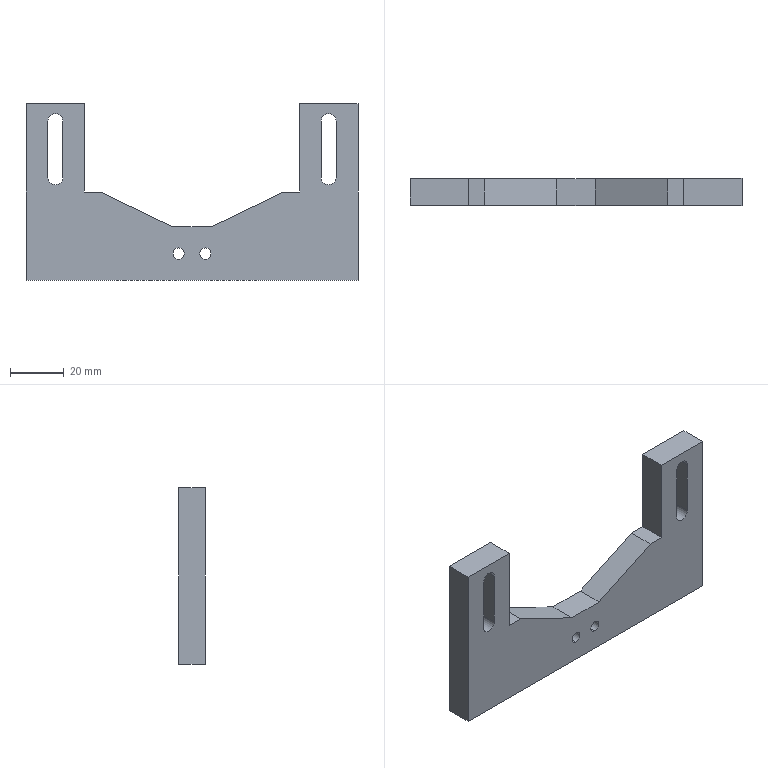Part | 1 solid | 28 faces | box 124 x 10 x 66 mm | volume 46758 mm3 | plane 18 | cylinder 10 | commonest cylinder face diameters 5.6 x6 4.2 x4
STEP:
#1=CARTESIAN_POINT('',(57.,0.,-58.1));
#2=VERTEX_POINT('',#1);
#3=CARTESIAN_POINT('',(57.,0.,-53.9));
#4=VERTEX_POINT('',#3);
#5=CARTESIAN_POINT('',(57.,0.,-56.));
#6=DIRECTION('',(0.,1.,0.));
#7=DIRECTION('',(0.,0.,1.));
#8=AXIS2_PLACEMENT_3D('',#5,#6,#7);
#9=CIRCLE('',#8,2.1);
#10=EDGE_CURVE('',#2,#4,#9,.T.);
#11=ORIENTED_EDGE('',*,*,#10,.F.);
#12=CARTESIAN_POINT('',(57.,10.,-58.1));
#13=VERTEX_POINT('',#12);
#14=CARTESIAN_POINT('',(57.,10.,-58.1));
#15=DIRECTION('',(0.,1.,0.));
#16=VECTOR('',#15,1000.);
#17=LINE('',#14,#16);
#18=EDGE_CURVE('',#2,#13,#17,.T.);
#19=ORIENTED_EDGE('',*,*,#18,.T.);
#20=CARTESIAN_POINT('',(57.,10.,-53.9));
#21=VERTEX_POINT('',#20);
#22=CARTESIAN_POINT('',(57.,10.,-56.));
#23=DIRECTION('',(0.,1.,0.));
#24=DIRECTION('',(0.,0.,1.));
#25=AXIS2_PLACEMENT_3D('',#22,#23,#24);
#26=CIRCLE('',#25,2.1);
#27=EDGE_CURVE('',#13,#21,#26,.T.);
#28=ORIENTED_EDGE('',*,*,#27,.T.);
#29=CARTESIAN_POINT('',(57.,10.,-53.9));
#30=DIRECTION('',(0.,1.,0.));
#31=VECTOR('',#30,1000.);
#32=LINE('',#29,#31);
#33=EDGE_CURVE('',#4,#21,#32,.T.);
#34=ORIENTED_EDGE('',*,*,#33,.F.);
#35=EDGE_LOOP('',(#11,#19,#28,#34));
#36=FACE_OUTER_BOUND('',#35,.T.);
#37=CARTESIAN_POINT('',(57.,10.,-56.));
#38=DIRECTION('',(0.,1.,0.));
#39=DIRECTION('',(0.,0.,1.));
#40=AXIS2_PLACEMENT_3D('',#37,#38,#39);
#41=CYLINDRICAL_SURFACE('',#40,2.1);
#42=ADVANCED_FACE('',(#36),#41,.F.);
#43=CARTESIAN_POINT('',(67.,0.,-58.1));
#44=VERTEX_POINT('',#43);
#45=CARTESIAN_POINT('',(67.,0.,-53.9));
#46=VERTEX_POINT('',#45);
#47=CARTESIAN_POINT('',(67.,0.,-56.));
#48=DIRECTION('',(0.,1.,0.));
#49=DIRECTION('',(0.,0.,1.));
#50=AXIS2_PLACEMENT_3D('',#47,#48,#49);
#51=CIRCLE('',#50,2.1);
#52=EDGE_CURVE('',#44,#46,#51,.T.);
#53=ORIENTED_EDGE('',*,*,#52,.F.);
#54=CARTESIAN_POINT('',(67.,10.,-58.1));
#55=VERTEX_POINT('',#54);
#56=CARTESIAN_POINT('',(67.,10.,-58.1));
#57=DIRECTION('',(0.,1.,0.));
#58=VECTOR('',#57,1000.);
#59=LINE('',#56,#58);
#60=EDGE_CURVE('',#44,#55,#59,.T.);
#61=ORIENTED_EDGE('',*,*,#60,.T.);
#62=CARTESIAN_POINT('',(67.,10.,-53.9));
#63=VERTEX_POINT('',#62);
#64=CARTESIAN_POINT('',(67.,10.,-56.));
#65=DIRECTION('',(0.,1.,0.));
#66=DIRECTION('',(0.,0.,1.));
#67=AXIS2_PLACEMENT_3D('',#64,#65,#66);
#68=CIRCLE('',#67,2.1);
#69=EDGE_CURVE('',#55,#63,#68,.T.);
#70=ORIENTED_EDGE('',*,*,#69,.T.);
#71=CARTESIAN_POINT('',(67.,10.,-53.9));
#72=DIRECTION('',(0.,1.,0.));
#73=VECTOR('',#72,1000.);
#74=LINE('',#71,#73);
#75=EDGE_CURVE('',#46,#63,#74,.T.);
#76=ORIENTED_EDGE('',*,*,#75,.F.);
#77=EDGE_LOOP('',(#53,#61,#70,#76));
#78=FACE_OUTER_BOUND('',#77,.T.);
#79=CARTESIAN_POINT('',(67.,10.,-56.));
#80=DIRECTION('',(0.,1.,0.));
#81=DIRECTION('',(0.,0.,1.));
#82=AXIS2_PLACEMENT_3D('',#79,#80,#81);
#83=CYLINDRICAL_SURFACE('',#82,2.1);
#84=ADVANCED_FACE('',(#78),#83,.F.);
#85=CARTESIAN_POINT('',(11.,0.,-3.7));
#86=VERTEX_POINT('',#85);
#87=CARTESIAN_POINT('',(13.8,0.,-6.5));
#88=VERTEX_POINT('',#87);
#89=CARTESIAN_POINT('',(11.,0.,-6.5));
#90=DIRECTION('',(0.,1.,0.));
#91=DIRECTION('',(0.,0.,1.));
#92=AXIS2_PLACEMENT_3D('',#89,#90,#91);
#93=CIRCLE('',#92,2.8);
#94=EDGE_CURVE('',#86,#88,#93,.T.);
#95=ORIENTED_EDGE('',*,*,#94,.F.);
#96=CARTESIAN_POINT('',(11.,10.,-3.7));
#97=VERTEX_POINT('',#96);
#98=CARTESIAN_POINT('',(11.,0.,-3.7));
#99=DIRECTION('',(0.,1.,0.));
#100=VECTOR('',#99,1000.);
#101=LINE('',#98,#100);
#102=EDGE_CURVE('',#86,#97,#101,.T.);
#103=ORIENTED_EDGE('',*,*,#102,.T.);
#104=CARTESIAN_POINT('',(13.8,10.,-6.5));
#105=VERTEX_POINT('',#104);
#106=CARTESIAN_POINT('',(11.,10.,-6.5));
#107=DIRECTION('',(0.,1.,0.));
#108=DIRECTION('',(0.,0.,1.));
#109=AXIS2_PLACEMENT_3D('',#106,#107,#108);
#110=CIRCLE('',#109,2.8);
#111=EDGE_CURVE('',#97,#105,#110,.T.);
#112=ORIENTED_EDGE('',*,*,#111,.T.);
#113=CARTESIAN_POINT('',(13.8,0.,-6.5));
#114=DIRECTION('',(0.,1.,0.));
#115=VECTOR('',#114,1000.);
#116=LINE('',#113,#115);
#117=EDGE_CURVE('',#88,#105,#116,.T.);
#118=ORIENTED_EDGE('',*,*,#117,.F.);
#119=EDGE_LOOP('',(#95,#103,#112,#118));
#120=FACE_OUTER_BOUND('',#119,.T.);
#121=CARTESIAN_POINT('',(11.,0.,-6.5));
#122=DIRECTION('',(0.,1.,0.));
#123=DIRECTION('',(0.,0.,1.));
#124=AXIS2_PLACEMENT_3D('',#121,#122,#123);
#125=CYLINDRICAL_SURFACE('',#124,2.8);
#126=ADVANCED_FACE('',(#120),#125,.F.);
#127=CARTESIAN_POINT('',(113.,0.,-3.7));
#128=VERTEX_POINT('',#127);
#129=CARTESIAN_POINT('',(115.8,0.,-6.5));
#130=VERTEX_POINT('',#129);
#131=CARTESIAN_POINT('',(113.,0.,-6.5));
#132=DIRECTION('',(0.,1.,0.));
#133=DIRECTION('',(0.,0.,-1.));
#134=AXIS2_PLACEMENT_3D('',#131,#132,#133);
#135=CIRCLE('',#134,2.8);
#136=EDGE_CURVE('',#128,#130,#135,.T.);
#137=ORIENTED_EDGE('',*,*,#136,.F.);
#138=CARTESIAN_POINT('',(113.,10.,-3.7));
#139=VERTEX_POINT('',#138);
#140=CARTESIAN_POINT('',(113.,0.,-3.7));
#141=DIRECTION('',(0.,1.,0.));
#142=VECTOR('',#141,1000.);
#143=LINE('',#140,#142);
#144=EDGE_CURVE('',#128,#139,#143,.T.);
#145=ORIENTED_EDGE('',*,*,#144,.T.);
#146=CARTESIAN_POINT('',(115.8,10.,-6.5));
#147=VERTEX_POINT('',#146);
#148=CARTESIAN_POINT('',(113.,10.,-6.5));
#149=DIRECTION('',(0.,1.,0.));
#150=DIRECTION('',(0.,0.,-1.));
#151=AXIS2_PLACEMENT_3D('',#148,#149,#150);
#152=CIRCLE('',#151,2.8);
#153=EDGE_CURVE('',#139,#147,#152,.T.);
#154=ORIENTED_EDGE('',*,*,#153,.T.);
#155=CARTESIAN_POINT('',(115.8,0.,-6.5));
#156=DIRECTION('',(0.,1.,0.));
#157=VECTOR('',#156,1000.);
#158=LINE('',#155,#157);
#159=EDGE_CURVE('',#130,#147,#158,.T.);
#160=ORIENTED_EDGE('',*,*,#159,.F.);
#161=EDGE_LOOP('',(#137,#145,#154,#160));
#162=FACE_OUTER_BOUND('',#161,.T.);
#163=CARTESIAN_POINT('',(113.,0.,-6.5));
#164=DIRECTION('',(0.,1.,0.));
#165=DIRECTION('',(0.,0.,1.));
#166=AXIS2_PLACEMENT_3D('',#163,#164,#165);
#167=CYLINDRICAL_SURFACE('',#166,2.8);
#168=ADVANCED_FACE('',(#162),#167,.F.);
#169=CARTESIAN_POINT('',(0.,0.,0.));
#170=VERTEX_POINT('',#169);
#171=CARTESIAN_POINT('',(21.75,0.,0.));
#172=VERTEX_POINT('',#171);
#173=CARTESIAN_POINT('',(0.,0.,0.));
#174=DIRECTION('',(1.,0.,0.));
#175=VECTOR('',#174,1000.);
#176=LINE('',#173,#175);
#177=EDGE_CURVE('',#170,#172,#176,.T.);
#178=ORIENTED_EDGE('',*,*,#177,.T.);
#179=CARTESIAN_POINT('',(21.75,10.,0.));
#180=VERTEX_POINT('',#179);
#181=CARTESIAN_POINT('',(21.75,10.,0.));
#182=DIRECTION('',(0.,-1.,0.));
#183=VECTOR('',#182,1000.);
#184=LINE('',#181,#183);
#185=EDGE_CURVE('',#180,#172,#184,.T.);
#186=ORIENTED_EDGE('',*,*,#185,.F.);
#187=CARTESIAN_POINT('',(0.,10.,0.));
#188=VERTEX_POINT('',#187);
#189=CARTESIAN_POINT('',(0.,10.,0.));
#190=DIRECTION('',(1.,0.,0.));
#191=VECTOR('',#190,1000.);
#192=LINE('',#189,#191);
#193=EDGE_CURVE('',#188,#180,#192,.T.);
#194=ORIENTED_EDGE('',*,*,#193,.F.);
#195=CARTESIAN_POINT('',(0.,10.,0.));
#196=DIRECTION('',(0.,-1.,0.));
#197=VECTOR('',#196,1000.);
#198=LINE('',#195,#197);
#199=EDGE_CURVE('',#188,#170,#198,.T.);
#200=ORIENTED_EDGE('',*,*,#199,.T.);
#201=EDGE_LOOP('',(#178,#186,#194,#200));
#202=FACE_OUTER_BOUND('',#201,.T.);
#203=CARTESIAN_POINT('',(0.,10.,0.));
#204=DIRECTION('',(0.,0.,-1.));
#205=DIRECTION('',(-1.,0.,0.));
#206=AXIS2_PLACEMENT_3D('',#203,#204,#205);
#207=PLANE('',#206);
#208=ADVANCED_FACE('',(#202),#207,.F.);
#209=CARTESIAN_POINT('',(21.75,0.,-33.));
#210=VERTEX_POINT('',#209);
#211=CARTESIAN_POINT('',(21.75,0.,0.));
#212=DIRECTION('',(0.,0.,-1.));
#213=VECTOR('',#212,1000.);
#214=LINE('',#211,#213);
#215=EDGE_CURVE('',#172,#210,#214,.T.);
#216=ORIENTED_EDGE('',*,*,#215,.T.);
#217=CARTESIAN_POINT('',(21.75,10.,-33.));
#218=VERTEX_POINT('',#217);
#219=CARTESIAN_POINT('',(21.75,10.,-33.));
#220=DIRECTION('',(0.,-1.,0.));
#221=VECTOR('',#220,1000.);
#222=LINE('',#219,#221);
#223=EDGE_CURVE('',#218,#210,#222,.T.);
#224=ORIENTED_EDGE('',*,*,#223,.F.);
#225=CARTESIAN_POINT('',(21.75,10.,0.));
#226=DIRECTION('',(0.,0.,-1.));
#227=VECTOR('',#226,1000.);
#228=LINE('',#225,#227);
#229=EDGE_CURVE('',#180,#218,#228,.T.);
#230=ORIENTED_EDGE('',*,*,#229,.F.);
#231=ORIENTED_EDGE('',*,*,#185,.T.);
#232=EDGE_LOOP('',(#216,#224,#230,#231));
#233=FACE_OUTER_BOUND('',#232,.T.);
#234=CARTESIAN_POINT('',(21.75,10.,0.));
#235=DIRECTION('',(-1.,0.,0.));
#236=DIRECTION('',(0.,0.,1.));
#237=AXIS2_PLACEMENT_3D('',#234,#235,#236);
#238=PLANE('',#237);
#239=ADVANCED_FACE('',(#233),#238,.F.);
#240=CARTESIAN_POINT('',(27.75,0.,-33.));
#241=VERTEX_POINT('',#240);
#242=CARTESIAN_POINT('',(21.75,0.,-33.));
#243=DIRECTION('',(1.,0.,0.));
#244=VECTOR('',#243,1000.);
#245=LINE('',#242,#244);
#246=EDGE_CURVE('',#210,#241,#245,.T.);
#247=ORIENTED_EDGE('',*,*,#246,.T.);
#248=CARTESIAN_POINT('',(27.75,10.,-33.));
#249=VERTEX_POINT('',#248);
#250=CARTESIAN_POINT('',(27.75,10.,-33.));
#251=DIRECTION('',(0.,-1.,0.));
#252=VECTOR('',#251,1000.);
#253=LINE('',#250,#252);
#254=EDGE_CURVE('',#249,#241,#253,.T.);
#255=ORIENTED_EDGE('',*,*,#254,.F.);
#256=CARTESIAN_POINT('',(21.75,10.,-33.));
#257=DIRECTION('',(1.,0.,0.));
#258=VECTOR('',#257,1000.);
#259=LINE('',#256,#258);
#260=EDGE_CURVE('',#218,#249,#259,.T.);
#261=ORIENTED_EDGE('',*,*,#260,.F.);
#262=ORIENTED_EDGE('',*,*,#223,.T.);
#263=EDGE_LOOP('',(#247,#255,#261,#262));
#264=FACE_OUTER_BOUND('',#263,.T.);
#265=CARTESIAN_POINT('',(21.75,10.,-33.));
#266=DIRECTION('',(0.,0.,-1.));
#267=DIRECTION('',(-1.,0.,0.));
#268=AXIS2_PLACEMENT_3D('',#265,#266,#267);
#269=PLANE('',#268);
#270=ADVANCED_FACE('',(#264),#269,.F.);
#271=CARTESIAN_POINT('',(54.75,0.,-46.));
#272=VERTEX_POINT('',#271);
#273=CARTESIAN_POINT('',(27.75,0.,-33.));
#274=DIRECTION('',(0.901,0.,-0.4338));
#275=VECTOR('',#274,1000.);
#276=LINE('',#273,#275);
#277=EDGE_CURVE('',#241,#272,#276,.T.);
#278=ORIENTED_EDGE('',*,*,#277,.T.);
#279=CARTESIAN_POINT('',(54.75,10.,-46.));
#280=VERTEX_POINT('',#279);
#281=CARTESIAN_POINT('',(54.75,10.,-46.));
#282=DIRECTION('',(0.,-1.,0.));
#283=VECTOR('',#282,1000.);
#284=LINE('',#281,#283);
#285=EDGE_CURVE('',#280,#272,#284,.T.);
#286=ORIENTED_EDGE('',*,*,#285,.F.);
#287=CARTESIAN_POINT('',(27.75,10.,-33.));
#288=DIRECTION('',(0.901,0.,-0.4338));
#289=VECTOR('',#288,1000.);
#290=LINE('',#287,#289);
#291=EDGE_CURVE('',#249,#280,#290,.T.);
#292=ORIENTED_EDGE('',*,*,#291,.F.);
#293=ORIENTED_EDGE('',*,*,#254,.T.);
#294=EDGE_LOOP('',(#278,#286,#292,#293));
#295=FACE_OUTER_BOUND('',#294,.T.);
#296=CARTESIAN_POINT('',(27.75,10.,-33.));
#297=DIRECTION('',(-0.4338,0.,-0.901));
#298=DIRECTION('',(-0.901,0.,0.4338));
#299=AXIS2_PLACEMENT_3D('',#296,#297,#298);
#300=PLANE('',#299);
#301=ADVANCED_FACE('',(#295),#300,.F.);
#302=CARTESIAN_POINT('',(69.25,0.,-46.));
#303=VERTEX_POINT('',#302);
#304=CARTESIAN_POINT('',(69.25,0.,-46.));
#305=DIRECTION('',(1.,0.,0.));
#306=VECTOR('',#305,1000.);
#307=LINE('',#304,#306);
#308=EDGE_CURVE('',#272,#303,#307,.T.);
#309=ORIENTED_EDGE('',*,*,#308,.T.);
#310=CARTESIAN_POINT('',(69.25,10.,-46.));
#311=VERTEX_POINT('',#310);
#312=CARTESIAN_POINT('',(69.25,10.,-46.));
#313=DIRECTION('',(0.,-1.,0.));
#314=VECTOR('',#313,1000.);
#315=LINE('',#312,#314);
#316=EDGE_CURVE('',#311,#303,#315,.T.);
#317=ORIENTED_EDGE('',*,*,#316,.F.);
#318=CARTESIAN_POINT('',(69.25,10.,-46.));
#319=DIRECTION('',(1.,0.,0.));
#320=VECTOR('',#319,1000.);
#321=LINE('',#318,#320);
#322=EDGE_CURVE('',#280,#311,#321,.T.);
#323=ORIENTED_EDGE('',*,*,#322,.F.);
#324=ORIENTED_EDGE('',*,*,#285,.T.);
#325=EDGE_LOOP('',(#309,#317,#323,#324));
#326=FACE_OUTER_BOUND('',#325,.T.);
#327=CARTESIAN_POINT('',(69.25,10.,-46.));
#328=DIRECTION('',(0.,0.,-1.));
#329=DIRECTION('',(-1.,0.,0.));
#330=AXIS2_PLACEMENT_3D('',#327,#328,#329);
#331=PLANE('',#330);
#332=ADVANCED_FACE('',(#326),#331,.F.);
#333=CARTESIAN_POINT('',(96.25,0.,-33.));
#334=VERTEX_POINT('',#333);
#335=CARTESIAN_POINT('',(96.25,0.,-33.));
#336=DIRECTION('',(0.901,0.,0.4338));
#337=VECTOR('',#336,1000.);
#338=LINE('',#335,#337);
#339=EDGE_CURVE('',#303,#334,#338,.T.);
#340=ORIENTED_EDGE('',*,*,#339,.T.);
#341=CARTESIAN_POINT('',(96.25,10.,-33.));
#342=VERTEX_POINT('',#341);
#343=CARTESIAN_POINT('',(96.25,10.,-33.));
#344=DIRECTION('',(0.,-1.,0.));
#345=VECTOR('',#344,1000.);
#346=LINE('',#343,#345);
#347=EDGE_CURVE('',#342,#334,#346,.T.);
#348=ORIENTED_EDGE('',*,*,#347,.F.);
#349=CARTESIAN_POINT('',(96.25,10.,-33.));
#350=DIRECTION('',(0.901,0.,0.4338));
#351=VECTOR('',#350,1000.);
#352=LINE('',#349,#351);
#353=EDGE_CURVE('',#311,#342,#352,.T.);
#354=ORIENTED_EDGE('',*,*,#353,.F.);
#355=ORIENTED_EDGE('',*,*,#316,.T.);
#356=EDGE_LOOP('',(#340,#348,#354,#355));
#357=FACE_OUTER_BOUND('',#356,.T.);
#358=CARTESIAN_POINT('',(96.25,10.,-33.));
#359=DIRECTION('',(0.4338,0.,-0.901));
#360=DIRECTION('',(-0.901,0.,-0.4338));
#361=AXIS2_PLACEMENT_3D('',#358,#359,#360);
#362=PLANE('',#361);
#363=ADVANCED_FACE('',(#357),#362,.F.);
#364=CARTESIAN_POINT('',(102.25,0.,-33.));
#365=VERTEX_POINT('',#364);
#366=CARTESIAN_POINT('',(102.25,0.,-33.));
#367=DIRECTION('',(1.,0.,0.));
#368=VECTOR('',#367,1000.);
#369=LINE('',#366,#368);
#370=EDGE_CURVE('',#334,#365,#369,.T.);
#371=ORIENTED_EDGE('',*,*,#370,.T.);
#372=CARTESIAN_POINT('',(102.25,10.,-33.));
#373=VERTEX_POINT('',#372);
#374=CARTESIAN_POINT('',(102.25,10.,-33.));
#375=DIRECTION('',(0.,-1.,0.));
#376=VECTOR('',#375,1000.);
#377=LINE('',#374,#376);
#378=EDGE_CURVE('',#373,#365,#377,.T.);
#379=ORIENTED_EDGE('',*,*,#378,.F.);
#380=CARTESIAN_POINT('',(102.25,10.,-33.));
#381=DIRECTION('',(1.,0.,0.));
#382=VECTOR('',#381,1000.);
#383=LINE('',#380,#382);
#384=EDGE_CURVE('',#342,#373,#383,.T.);
#385=ORIENTED_EDGE('',*,*,#384,.F.);
#386=ORIENTED_EDGE('',*,*,#347,.T.);
#387=EDGE_LOOP('',(#371,#379,#385,#386));
#388=FACE_OUTER_BOUND('',#387,.T.);
#389=CARTESIAN_POINT('',(102.25,10.,-33.));
#390=DIRECTION('',(0.,0.,-1.));
#391=DIRECTION('',(-1.,0.,0.));
#392=AXIS2_PLACEMENT_3D('',#389,#390,#391);
#393=PLANE('',#392);
#394=ADVANCED_FACE('',(#388),#393,.F.);
#395=CARTESIAN_POINT('',(102.25,0.,0.));
#396=VERTEX_POINT('',#395);
#397=CARTESIAN_POINT('',(102.25,0.,0.));
#398=DIRECTION('',(0.,0.,1.));
#399=VECTOR('',#398,1000.);
#400=LINE('',#397,#399);
#401=EDGE_CURVE('',#365,#396,#400,.T.);
#402=ORIENTED_EDGE('',*,*,#401,.T.);
#403=CARTESIAN_POINT('',(102.25,10.,0.));
#404=VERTEX_POINT('',#403);
#405=CARTESIAN_POINT('',(102.25,10.,0.));
#406=DIRECTION('',(0.,-1.,0.));
#407=VECTOR('',#406,1000.);
#408=LINE('',#405,#407);
#409=EDGE_CURVE('',#404,#396,#408,.T.);
#410=ORIENTED_EDGE('',*,*,#409,.F.);
#411=CARTESIAN_POINT('',(102.25,10.,0.));
#412=DIRECTION('',(0.,0.,1.));
#413=VECTOR('',#412,1000.);
#414=LINE('',#411,#413);
#415=EDGE_CURVE('',#373,#404,#414,.T.);
#416=ORIENTED_EDGE('',*,*,#415,.F.);
#417=ORIENTED_EDGE('',*,*,#378,.T.);
#418=EDGE_LOOP('',(#402,#410,#416,#417));
#419=FACE_OUTER_BOUND('',#418,.T.);
#420=CARTESIAN_POINT('',(102.25,10.,0.));
#421=DIRECTION('',(1.,0.,0.));
#422=DIRECTION('',(0.,0.,-1.));
#423=AXIS2_PLACEMENT_3D('',#420,#421,#422);
#424=PLANE('',#423);
#425=ADVANCED_FACE('',(#419),#424,.F.);
#426=CARTESIAN_POINT('',(124.,0.,0.));
#427=VERTEX_POINT('',#426);
#428=CARTESIAN_POINT('',(124.,0.,0.));
#429=DIRECTION('',(1.,0.,0.));
#430=VECTOR('',#429,1000.);
#431=LINE('',#428,#430);
#432=EDGE_CURVE('',#396,#427,#431,.T.);
#433=ORIENTED_EDGE('',*,*,#432,.T.);
#434=CARTESIAN_POINT('',(124.,10.,0.));
#435=VERTEX_POINT('',#434);
#436=CARTESIAN_POINT('',(124.,10.,0.));
#437=DIRECTION('',(0.,-1.,0.));
#438=VECTOR('',#437,1000.);
#439=LINE('',#436,#438);
#440=EDGE_CURVE('',#435,#427,#439,.T.);
#441=ORIENTED_EDGE('',*,*,#440,.F.);
#442=CARTESIAN_POINT('',(124.,10.,0.));
#443=DIRECTION('',(1.,0.,0.));
#444=VECTOR('',#443,1000.);
#445=LINE('',#442,#444);
#446=EDGE_CURVE('',#404,#435,#445,.T.);
#447=ORIENTED_EDGE('',*,*,#446,.F.);
#448=ORIENTED_EDGE('',*,*,#409,.T.);
#449=EDGE_LOOP('',(#433,#441,#447,#448));
#450=FACE_OUTER_BOUND('',#449,.T.);
#451=CARTESIAN_POINT('',(124.,10.,0.));
#452=DIRECTION('',(0.,0.,-1.));
#453=DIRECTION('',(-1.,0.,0.));
#454=AXIS2_PLACEMENT_3D('',#451,#452,#453);
#455=PLANE('',#454);
#456=ADVANCED_FACE('',(#450),#455,.F.);
#457=CARTESIAN_POINT('',(124.,0.,-66.));
#458=VERTEX_POINT('',#457);
#459=CARTESIAN_POINT('',(124.,0.,-66.));
#460=DIRECTION('',(0.,0.,-1.));
#461=VECTOR('',#460,1000.);
#462=LINE('',#459,#461);
#463=EDGE_CURVE('',#427,#458,#462,.T.);
#464=ORIENTED_EDGE('',*,*,#463,.T.);
#465=CARTESIAN_POINT('',(124.,10.,-66.));
#466=VERTEX_POINT('',#465);
#467=CARTESIAN_POINT('',(124.,10.,-66.));
#468=DIRECTION('',(0.,-1.,0.));
#469=VECTOR('',#468,1000.);
#470=LINE('',#467,#469);
#471=EDGE_CURVE('',#466,#458,#470,.T.);
#472=ORIENTED_EDGE('',*,*,#471,.F.);
#473=CARTESIAN_POINT('',(124.,10.,-66.));
#474=DIRECTION('',(0.,0.,-1.));
#475=VECTOR('',#474,1000.);
#476=LINE('',#473,#475);
#477=EDGE_CURVE('',#435,#466,#476,.T.);
#478=ORIENTED_EDGE('',*,*,#477,.F.);
#479=ORIENTED_EDGE('',*,*,#440,.T.);
#480=EDGE_LOOP('',(#464,#472,#478,#479));
#481=FACE_OUTER_BOUND('',#480,.T.);
#482=CARTESIAN_POINT('',(124.,10.,-66.));
#483=DIRECTION('',(-1.,0.,0.));
#484=DIRECTION('',(0.,0.,1.));
#485=AXIS2_PLACEMENT_3D('',#482,#483,#484);
#486=PLANE('',#485);
#487=ADVANCED_FACE('',(#481),#486,.F.);
#488=CARTESIAN_POINT('',(0.,0.,-66.));
#489=VERTEX_POINT('',#488);
#490=CARTESIAN_POINT('',(0.,0.,-66.));
#491=DIRECTION('',(-1.,0.,0.));
#492=VECTOR('',#491,1000.);
#493=LINE('',#490,#492);
#494=EDGE_CURVE('',#458,#489,#493,.T.);
#495=ORIENTED_EDGE('',*,*,#494,.T.);
#496=CARTESIAN_POINT('',(0.,10.,-66.));
#497=VERTEX_POINT('',#496);
#498=CARTESIAN_POINT('',(0.,10.,-66.));
#499=DIRECTION('',(0.,-1.,0.));
#500=VECTOR('',#499,1000.);
#501=LINE('',#498,#500);
#502=EDGE_CURVE('',#497,#489,#501,.T.);
#503=ORIENTED_EDGE('',*,*,#502,.F.);
#504=CARTESIAN_POINT('',(0.,10.,-66.));
#505=DIRECTION('',(-1.,0.,0.));
#506=VECTOR('',#505,1000.);
#507=LINE('',#504,#506);
#508=EDGE_CURVE('',#466,#497,#507,.T.);
#509=ORIENTED_EDGE('',*,*,#508,.F.);
#510=ORIENTED_EDGE('',*,*,#471,.T.);
#511=EDGE_LOOP('',(#495,#503,#509,#510));
#512=FACE_OUTER_BOUND('',#511,.T.);
#513=CARTESIAN_POINT('',(0.,10.,-66.));
#514=DIRECTION('',(0.,0.,1.));
#515=DIRECTION('',(1.,0.,0.));
#516=AXIS2_PLACEMENT_3D('',#513,#514,#515);
#517=PLANE('',#516);
#518=ADVANCED_FACE('',(#512),#517,.F.);
#519=CARTESIAN_POINT('',(0.,0.,0.));
#520=DIRECTION('',(0.,0.,1.));
#521=VECTOR('',#520,1000.);
#522=LINE('',#519,#521);
#523=EDGE_CURVE('',#489,#170,#522,.T.);
#524=ORIENTED_EDGE('',*,*,#523,.T.);
#525=ORIENTED_EDGE('',*,*,#199,.F.);
#526=CARTESIAN_POINT('',(0.,10.,0.));
#527=DIRECTION('',(0.,0.,1.));
#528=VECTOR('',#527,1000.);
#529=LINE('',#526,#528);
#530=EDGE_CURVE('',#497,#188,#529,.T.);
#531=ORIENTED_EDGE('',*,*,#530,.F.);
#532=ORIENTED_EDGE('',*,*,#502,.T.);
#533=EDGE_LOOP('',(#524,#525,#531,#532));
#534=FACE_OUTER_BOUND('',#533,.T.);
#535=CARTESIAN_POINT('',(0.,10.,0.));
#536=DIRECTION('',(1.,0.,0.));
#537=DIRECTION('',(0.,0.,-1.));
#538=AXIS2_PLACEMENT_3D('',#535,#536,#537);
#539=PLANE('',#538);
#540=ADVANCED_FACE('',(#534),#539,.F.);
#541=CARTESIAN_POINT('',(57.,10.,-56.));
#542=DIRECTION('',(0.,1.,0.));
#543=DIRECTION('',(0.,0.,1.));
#544=AXIS2_PLACEMENT_3D('',#541,#542,#543);
#545=CIRCLE('',#544,2.1);
#546=EDGE_CURVE('',#21,#13,#545,.T.);
#547=ORIENTED_EDGE('',*,*,#546,.F.);
#548=ORIENTED_EDGE('',*,*,#27,.F.);
#549=EDGE_LOOP('',(#547,#548));
#550=FACE_BOUND('',#549,.T.);
#551=CARTESIAN_POINT('',(67.,10.,-56.));
#552=DIRECTION('',(0.,1.,0.));
#553=DIRECTION('',(0.,0.,1.));
#554=AXIS2_PLACEMENT_3D('',#551,#552,#553);
#555=CIRCLE('',#554,2.1);
#556=EDGE_CURVE('',#63,#55,#555,.T.);
#557=ORIENTED_EDGE('',*,*,#556,.F.);
#558=ORIENTED_EDGE('',*,*,#69,.F.);
#559=EDGE_LOOP('',(#557,#558));
#560=FACE_BOUND('',#559,.T.);
#561=CARTESIAN_POINT('',(8.2,10.,-6.5));
#562=VERTEX_POINT('',#561);
#563=CARTESIAN_POINT('',(11.,10.,-6.5));
#564=DIRECTION('',(0.,1.,0.));
#565=DIRECTION('',(0.,0.,1.));
#566=AXIS2_PLACEMENT_3D('',#563,#564,#565);
#567=CIRCLE('',#566,2.8);
#568=EDGE_CURVE('',#562,#97,#567,.T.);
#569=ORIENTED_EDGE('',*,*,#568,.F.);
#570=CARTESIAN_POINT('',(8.2,10.,-27.5));
#571=VERTEX_POINT('',#570);
#572=CARTESIAN_POINT('',(8.2,10.,-6.5));
#573=DIRECTION('',(0.,0.,1.));
#574=VECTOR('',#573,1000.);
#575=LINE('',#572,#574);
#576=EDGE_CURVE('',#571,#562,#575,.T.);
#577=ORIENTED_EDGE('',*,*,#576,.F.);
#578=CARTESIAN_POINT('',(13.8,10.,-27.5));
#579=VERTEX_POINT('',#578);
#580=CARTESIAN_POINT('',(11.,10.,-27.5));
#581=DIRECTION('',(0.,1.,0.));
#582=DIRECTION('',(0.,0.,1.));
#583=AXIS2_PLACEMENT_3D('',#580,#581,#582);
#584=CIRCLE('',#583,2.8);
#585=EDGE_CURVE('',#579,#571,#584,.T.);
#586=ORIENTED_EDGE('',*,*,#585,.F.);
#587=CARTESIAN_POINT('',(13.8,10.,-6.5));
#588=DIRECTION('',(0.,0.,-1.));
#589=VECTOR('',#588,1000.);
#590=LINE('',#587,#589);
#591=EDGE_CURVE('',#105,#579,#590,.T.);
#592=ORIENTED_EDGE('',*,*,#591,.F.);
#593=ORIENTED_EDGE('',*,*,#111,.F.);
#594=EDGE_LOOP('',(#569,#577,#586,#592,#593));
#595=FACE_BOUND('',#594,.T.);
#596=CARTESIAN_POINT('',(110.2,10.,-6.5));
#597=VERTEX_POINT('',#596);
#598=CARTESIAN_POINT('',(113.,10.,-6.5));
#599=DIRECTION('',(0.,1.,0.));
#600=DIRECTION('',(0.,0.,-1.));
#601=AXIS2_PLACEMENT_3D('',#598,#599,#600);
#602=CIRCLE('',#601,2.8);
#603=EDGE_CURVE('',#597,#139,#602,.T.);
#604=ORIENTED_EDGE('',*,*,#603,.F.);
#605=CARTESIAN_POINT('',(110.2,10.,-27.5));
#606=VERTEX_POINT('',#605);
#607=CARTESIAN_POINT('',(110.2,10.,-6.5));
#608=DIRECTION('',(0.,0.,1.));
#609=VECTOR('',#608,1000.);
#610=LINE('',#607,#609);
#611=EDGE_CURVE('',#606,#597,#610,.T.);
#612=ORIENTED_EDGE('',*,*,#611,.F.);
#613=CARTESIAN_POINT('',(115.8,10.,-27.5));
#614=VERTEX_POINT('',#613);
#615=CARTESIAN_POINT('',(113.,10.,-27.5));
#616=DIRECTION('',(0.,1.,0.));
#617=DIRECTION('',(0.,0.,-1.));
#618=AXIS2_PLACEMENT_3D('',#615,#616,#617);
#619=CIRCLE('',#618,2.8);
#620=EDGE_CURVE('',#614,#606,#619,.T.);
#621=ORIENTED_EDGE('',*,*,#620,.F.);
#622=CARTESIAN_POINT('',(115.8,10.,-6.5));
#623=DIRECTION('',(0.,0.,-1.));
#624=VECTOR('',#623,1000.);
#625=LINE('',#622,#624);
#626=EDGE_CURVE('',#147,#614,#625,.T.);
#627=ORIENTED_EDGE('',*,*,#626,.F.);
#628=ORIENTED_EDGE('',*,*,#153,.F.);
#629=EDGE_LOOP('',(#604,#612,#621,#627,#628));
#630=FACE_BOUND('',#629,.T.);
#631=ORIENTED_EDGE('',*,*,#193,.T.);
#632=ORIENTED_EDGE('',*,*,#229,.T.);
#633=ORIENTED_EDGE('',*,*,#260,.T.);
#634=ORIENTED_EDGE('',*,*,#291,.T.);
#635=ORIENTED_EDGE('',*,*,#322,.T.);
#636=ORIENTED_EDGE('',*,*,#353,.T.);
#637=ORIENTED_EDGE('',*,*,#384,.T.);
#638=ORIENTED_EDGE('',*,*,#415,.T.);
#639=ORIENTED_EDGE('',*,*,#446,.T.);
#640=ORIENTED_EDGE('',*,*,#477,.T.);
#641=ORIENTED_EDGE('',*,*,#508,.T.);
#642=ORIENTED_EDGE('',*,*,#530,.T.);
#643=EDGE_LOOP('',(#631,#632,#633,#634,#635,#636,#637,#638,#639,#640,#641,#642));
#644=FACE_OUTER_BOUND('',#643,.T.);
#645=CARTESIAN_POINT('',(0.,10.,0.));
#646=DIRECTION('',(0.,1.,0.));
#647=DIRECTION('',(0.,0.,1.));
#648=AXIS2_PLACEMENT_3D('',#645,#646,#647);
#649=PLANE('',#648);
#650=ADVANCED_FACE('',(#550,#560,#595,#630,#644),#649,.T.);
#651=CARTESIAN_POINT('',(57.,0.,-56.));
#652=DIRECTION('',(0.,1.,0.));
#653=DIRECTION('',(0.,0.,1.));
#654=AXIS2_PLACEMENT_3D('',#651,#652,#653);
#655=CIRCLE('',#654,2.1);
#656=EDGE_CURVE('',#4,#2,#655,.T.);
#657=ORIENTED_EDGE('',*,*,#656,.T.);
#658=ORIENTED_EDGE('',*,*,#10,.T.);
#659=EDGE_LOOP('',(#657,#658));
#660=FACE_BOUND('',#659,.T.);
#661=CARTESIAN_POINT('',(67.,0.,-56.));
#662=DIRECTION('',(0.,1.,0.));
#663=DIRECTION('',(0.,0.,1.));
#664=AXIS2_PLACEMENT_3D('',#661,#662,#663);
#665=CIRCLE('',#664,2.1);
#666=EDGE_CURVE('',#46,#44,#665,.T.);
#667=ORIENTED_EDGE('',*,*,#666,.T.);
#668=ORIENTED_EDGE('',*,*,#52,.T.);
#669=EDGE_LOOP('',(#667,#668));
#670=FACE_BOUND('',#669,.T.);
#671=CARTESIAN_POINT('',(8.2,0.,-27.5));
#672=VERTEX_POINT('',#671);
#673=CARTESIAN_POINT('',(8.2,0.,-6.5));
#674=VERTEX_POINT('',#673);
#675=CARTESIAN_POINT('',(8.2,0.,-6.5));
#676=DIRECTION('',(0.,0.,1.));
#677=VECTOR('',#676,1000.);
#678=LINE('',#675,#677);
#679=EDGE_CURVE('',#672,#674,#678,.T.);
#680=ORIENTED_EDGE('',*,*,#679,.T.);
#681=CARTESIAN_POINT('',(11.,0.,-6.5));
#682=DIRECTION('',(0.,1.,0.));
#683=DIRECTION('',(0.,0.,1.));
#684=AXIS2_PLACEMENT_3D('',#681,#682,#683);
#685=CIRCLE('',#684,2.8);
#686=EDGE_CURVE('',#674,#86,#685,.T.);
#687=ORIENTED_EDGE('',*,*,#686,.T.);
#688=ORIENTED_EDGE('',*,*,#94,.T.);
#689=CARTESIAN_POINT('',(13.8,0.,-27.5));
#690=VERTEX_POINT('',#689);
#691=CARTESIAN_POINT('',(13.8,0.,-6.5));
#692=DIRECTION('',(0.,0.,-1.));
#693=VECTOR('',#692,1000.);
#694=LINE('',#691,#693);
#695=EDGE_CURVE('',#88,#690,#694,.T.);
#696=ORIENTED_EDGE('',*,*,#695,.T.);
#697=CARTESIAN_POINT('',(11.,0.,-27.5));
#698=DIRECTION('',(0.,1.,0.));
#699=DIRECTION('',(0.,0.,1.));
#700=AXIS2_PLACEMENT_3D('',#697,#698,#699);
#701=CIRCLE('',#700,2.8);
#702=EDGE_CURVE('',#690,#672,#701,.T.);
#703=ORIENTED_EDGE('',*,*,#702,.T.);
#704=EDGE_LOOP('',(#680,#687,#688,#696,#703));
#705=FACE_BOUND('',#704,.T.);
#706=CARTESIAN_POINT('',(110.2,0.,-27.5));
#707=VERTEX_POINT('',#706);
#708=CARTESIAN_POINT('',(110.2,0.,-6.5));
#709=VERTEX_POINT('',#708);
#710=CARTESIAN_POINT('',(110.2,0.,-6.5));
#711=DIRECTION('',(0.,0.,1.));
#712=VECTOR('',#711,1000.);
#713=LINE('',#710,#712);
#714=EDGE_CURVE('',#707,#709,#713,.T.);
#715=ORIENTED_EDGE('',*,*,#714,.T.);
#716=CARTESIAN_POINT('',(113.,0.,-6.5));
#717=DIRECTION('',(0.,1.,0.));
#718=DIRECTION('',(0.,0.,-1.));
#719=AXIS2_PLACEMENT_3D('',#716,#717,#718);
#720=CIRCLE('',#719,2.8);
#721=EDGE_CURVE('',#709,#128,#720,.T.);
#722=ORIENTED_EDGE('',*,*,#721,.T.);
#723=ORIENTED_EDGE('',*,*,#136,.T.);
#724=CARTESIAN_POINT('',(115.8,0.,-27.5));
#725=VERTEX_POINT('',#724);
#726=CARTESIAN_POINT('',(115.8,0.,-6.5));
#727=DIRECTION('',(0.,0.,-1.));
#728=VECTOR('',#727,1000.);
#729=LINE('',#726,#728);
#730=EDGE_CURVE('',#130,#725,#729,.T.);
#731=ORIENTED_EDGE('',*,*,#730,.T.);
#732=CARTESIAN_POINT('',(113.,0.,-27.5));
#733=DIRECTION('',(0.,1.,0.));
#734=DIRECTION('',(0.,0.,-1.));
#735=AXIS2_PLACEMENT_3D('',#732,#733,#734);
#736=CIRCLE('',#735,2.8);
#737=EDGE_CURVE('',#725,#707,#736,.T.);
#738=ORIENTED_EDGE('',*,*,#737,.T.);
#739=EDGE_LOOP('',(#715,#722,#723,#731,#738));
#740=FACE_BOUND('',#739,.T.);
#741=ORIENTED_EDGE('',*,*,#177,.F.);
#742=ORIENTED_EDGE('',*,*,#523,.F.);
#743=ORIENTED_EDGE('',*,*,#494,.F.);
#744=ORIENTED_EDGE('',*,*,#463,.F.);
#745=ORIENTED_EDGE('',*,*,#432,.F.);
#746=ORIENTED_EDGE('',*,*,#401,.F.);
#747=ORIENTED_EDGE('',*,*,#370,.F.);
#748=ORIENTED_EDGE('',*,*,#339,.F.);
#749=ORIENTED_EDGE('',*,*,#308,.F.);
#750=ORIENTED_EDGE('',*,*,#277,.F.);
#751=ORIENTED_EDGE('',*,*,#246,.F.);
#752=ORIENTED_EDGE('',*,*,#215,.F.);
#753=EDGE_LOOP('',(#741,#742,#743,#744,#745,#746,#747,#748,#749,#750,#751,#752));
#754=FACE_OUTER_BOUND('',#753,.T.);
#755=CARTESIAN_POINT('',(0.,0.,0.));
#756=DIRECTION('',(0.,1.,0.));
#757=DIRECTION('',(0.,0.,1.));
#758=AXIS2_PLACEMENT_3D('',#755,#756,#757);
#759=PLANE('',#758);
#760=ADVANCED_FACE('',(#660,#670,#705,#740,#754),#759,.F.);
#761=ORIENTED_EDGE('',*,*,#144,.F.);
#762=ORIENTED_EDGE('',*,*,#721,.F.);
#763=CARTESIAN_POINT('',(110.2,0.,-6.5));
#764=DIRECTION('',(0.,1.,0.));
#765=VECTOR('',#764,1000.);
#766=LINE('',#763,#765);
#767=EDGE_CURVE('',#709,#597,#766,.T.);
#768=ORIENTED_EDGE('',*,*,#767,.T.);
#769=ORIENTED_EDGE('',*,*,#603,.T.);
#770=EDGE_LOOP('',(#761,#762,#768,#769));
#771=FACE_OUTER_BOUND('',#770,.T.);
#772=CARTESIAN_POINT('',(113.,0.,-6.5));
#773=DIRECTION('',(0.,1.,0.));
#774=DIRECTION('',(0.,0.,1.));
#775=AXIS2_PLACEMENT_3D('',#772,#773,#774);
#776=CYLINDRICAL_SURFACE('',#775,2.8);
#777=ADVANCED_FACE('',(#771),#776,.F.);
#778=ORIENTED_EDGE('',*,*,#611,.T.);
#779=ORIENTED_EDGE('',*,*,#767,.F.);
#780=ORIENTED_EDGE('',*,*,#714,.F.);
#781=CARTESIAN_POINT('',(110.2,0.,-27.5));
#782=DIRECTION('',(0.,1.,0.));
#783=VECTOR('',#782,1000.);
#784=LINE('',#781,#783);
#785=EDGE_CURVE('',#707,#606,#784,.T.);
#786=ORIENTED_EDGE('',*,*,#785,.T.);
#787=EDGE_LOOP('',(#778,#779,#780,#786));
#788=FACE_OUTER_BOUND('',#787,.T.);
#789=CARTESIAN_POINT('',(110.2,0.,-6.5));
#790=DIRECTION('',(-1.,0.,0.));
#791=DIRECTION('',(0.,0.,1.));
#792=AXIS2_PLACEMENT_3D('',#789,#790,#791);
#793=PLANE('',#792);
#794=ADVANCED_FACE('',(#788),#793,.F.);
#795=ORIENTED_EDGE('',*,*,#620,.T.);
#796=ORIENTED_EDGE('',*,*,#785,.F.);
#797=ORIENTED_EDGE('',*,*,#737,.F.);
#798=CARTESIAN_POINT('',(115.8,0.,-27.5));
#799=DIRECTION('',(0.,1.,0.));
#800=VECTOR('',#799,1000.);
#801=LINE('',#798,#800);
#802=EDGE_CURVE('',#725,#614,#801,.T.);
#803=ORIENTED_EDGE('',*,*,#802,.T.);
#804=EDGE_LOOP('',(#795,#796,#797,#803));
#805=FACE_OUTER_BOUND('',#804,.T.);
#806=CARTESIAN_POINT('',(113.,0.,-27.5));
#807=DIRECTION('',(0.,1.,0.));
#808=DIRECTION('',(0.,0.,1.));
#809=AXIS2_PLACEMENT_3D('',#806,#807,#808);
#810=CYLINDRICAL_SURFACE('',#809,2.8);
#811=ADVANCED_FACE('',(#805),#810,.F.);
#812=ORIENTED_EDGE('',*,*,#626,.T.);
#813=ORIENTED_EDGE('',*,*,#802,.F.);
#814=ORIENTED_EDGE('',*,*,#730,.F.);
#815=ORIENTED_EDGE('',*,*,#159,.T.);
#816=EDGE_LOOP('',(#812,#813,#814,#815));
#817=FACE_OUTER_BOUND('',#816,.T.);
#818=CARTESIAN_POINT('',(115.8,0.,-6.5));
#819=DIRECTION('',(1.,0.,0.));
#820=DIRECTION('',(0.,0.,-1.));
#821=AXIS2_PLACEMENT_3D('',#818,#819,#820);
#822=PLANE('',#821);
#823=ADVANCED_FACE('',(#817),#822,.F.);
#824=ORIENTED_EDGE('',*,*,#102,.F.);
#825=ORIENTED_EDGE('',*,*,#686,.F.);
#826=CARTESIAN_POINT('',(8.2,0.,-6.5));
#827=DIRECTION('',(0.,1.,0.));
#828=VECTOR('',#827,1000.);
#829=LINE('',#826,#828);
#830=EDGE_CURVE('',#674,#562,#829,.T.);
#831=ORIENTED_EDGE('',*,*,#830,.T.);
#832=ORIENTED_EDGE('',*,*,#568,.T.);
#833=EDGE_LOOP('',(#824,#825,#831,#832));
#834=FACE_OUTER_BOUND('',#833,.T.);
#835=CARTESIAN_POINT('',(11.,0.,-6.5));
#836=DIRECTION('',(0.,1.,0.));
#837=DIRECTION('',(0.,0.,1.));
#838=AXIS2_PLACEMENT_3D('',#835,#836,#837);
#839=CYLINDRICAL_SURFACE('',#838,2.8);
#840=ADVANCED_FACE('',(#834),#839,.F.);
#841=ORIENTED_EDGE('',*,*,#576,.T.);
#842=ORIENTED_EDGE('',*,*,#830,.F.);
#843=ORIENTED_EDGE('',*,*,#679,.F.);
#844=CARTESIAN_POINT('',(8.2,0.,-27.5));
#845=DIRECTION('',(0.,1.,0.));
#846=VECTOR('',#845,1000.);
#847=LINE('',#844,#846);
#848=EDGE_CURVE('',#672,#571,#847,.T.);
#849=ORIENTED_EDGE('',*,*,#848,.T.);
#850=EDGE_LOOP('',(#841,#842,#843,#849));
#851=FACE_OUTER_BOUND('',#850,.T.);
#852=CARTESIAN_POINT('',(8.2,0.,-6.5));
#853=DIRECTION('',(-1.,0.,0.));
#854=DIRECTION('',(0.,0.,1.));
#855=AXIS2_PLACEMENT_3D('',#852,#853,#854);
#856=PLANE('',#855);
#857=ADVANCED_FACE('',(#851),#856,.F.);
#858=ORIENTED_EDGE('',*,*,#585,.T.);
#859=ORIENTED_EDGE('',*,*,#848,.F.);
#860=ORIENTED_EDGE('',*,*,#702,.F.);
#861=CARTESIAN_POINT('',(13.8,0.,-27.5));
#862=DIRECTION('',(0.,1.,0.));
#863=VECTOR('',#862,1000.);
#864=LINE('',#861,#863);
#865=EDGE_CURVE('',#690,#579,#864,.T.);
#866=ORIENTED_EDGE('',*,*,#865,.T.);
#867=EDGE_LOOP('',(#858,#859,#860,#866));
#868=FACE_OUTER_BOUND('',#867,.T.);
#869=CARTESIAN_POINT('',(11.,0.,-27.5));
#870=DIRECTION('',(0.,1.,0.));
#871=DIRECTION('',(0.,0.,1.));
#872=AXIS2_PLACEMENT_3D('',#869,#870,#871);
#873=CYLINDRICAL_SURFACE('',#872,2.8);
#874=ADVANCED_FACE('',(#868),#873,.F.);
#875=ORIENTED_EDGE('',*,*,#591,.T.);
#876=ORIENTED_EDGE('',*,*,#865,.F.);
#877=ORIENTED_EDGE('',*,*,#695,.F.);
#878=ORIENTED_EDGE('',*,*,#117,.T.);
#879=EDGE_LOOP('',(#875,#876,#877,#878));
#880=FACE_OUTER_BOUND('',#879,.T.);
#881=CARTESIAN_POINT('',(13.8,0.,-6.5));
#882=DIRECTION('',(1.,0.,0.));
#883=DIRECTION('',(0.,0.,-1.));
#884=AXIS2_PLACEMENT_3D('',#881,#882,#883);
#885=PLANE('',#884);
#886=ADVANCED_FACE('',(#880),#885,.F.);
#887=ORIENTED_EDGE('',*,*,#60,.F.);
#888=ORIENTED_EDGE('',*,*,#666,.F.);
#889=ORIENTED_EDGE('',*,*,#75,.T.);
#890=ORIENTED_EDGE('',*,*,#556,.T.);
#891=EDGE_LOOP('',(#887,#888,#889,#890));
#892=FACE_OUTER_BOUND('',#891,.T.);
#893=CARTESIAN_POINT('',(67.,10.,-56.));
#894=DIRECTION('',(0.,1.,0.));
#895=DIRECTION('',(0.,0.,1.));
#896=AXIS2_PLACEMENT_3D('',#893,#894,#895);
#897=CYLINDRICAL_SURFACE('',#896,2.1);
#898=ADVANCED_FACE('',(#892),#897,.F.);
#899=ORIENTED_EDGE('',*,*,#18,.F.);
#900=ORIENTED_EDGE('',*,*,#656,.F.);
#901=ORIENTED_EDGE('',*,*,#33,.T.);
#902=ORIENTED_EDGE('',*,*,#546,.T.);
#903=EDGE_LOOP('',(#899,#900,#901,#902));
#904=FACE_OUTER_BOUND('',#903,.T.);
#905=CARTESIAN_POINT('',(57.,10.,-56.));
#906=DIRECTION('',(0.,1.,0.));
#907=DIRECTION('',(0.,0.,1.));
#908=AXIS2_PLACEMENT_3D('',#905,#906,#907);
#909=CYLINDRICAL_SURFACE('',#908,2.1);
#910=ADVANCED_FACE('',(#904),#909,.F.);
#911=CLOSED_SHELL('',(#42,#84,#126,#168,#208,#239,#270,#301,#332,#363,#394,#425,#456,#487,#518,#540,#650,#760,#777,#794,#811,#823,#840,#857,#874,#886,#898,#910));
#912=MANIFOLD_SOLID_BREP('',#911);
#913=CARTESIAN_POINT('',(0.,0.,0.));
#914=DIRECTION('',(0.,0.,1.));
#915=DIRECTION('',(1.,0.,0.));
#916=AXIS2_PLACEMENT_3D('',#913,#914,#915);
#917=(LENGTH_UNIT()NAMED_UNIT(*)SI_UNIT(.MILLI.,.METRE.));
#918=UNCERTAINTY_MEASURE_WITH_UNIT(LENGTH_MEASURE(0.00001),#917,'','');
#919=(NAMED_UNIT(*)PLANE_ANGLE_UNIT()SI_UNIT($,.RADIAN.));
#920=(NAMED_UNIT(*)SI_UNIT($,.STERADIAN.)SOLID_ANGLE_UNIT());
#921=(GEOMETRIC_REPRESENTATION_CONTEXT(3)GLOBAL_UNCERTAINTY_ASSIGNED_CONTEXT((#918))GLOBAL_UNIT_ASSIGNED_CONTEXT((#917,#919,#920))REPRESENTATION_CONTEXT('',''));
#922=ADVANCED_BREP_SHAPE_REPRESENTATION('',(#912,#916),#921);